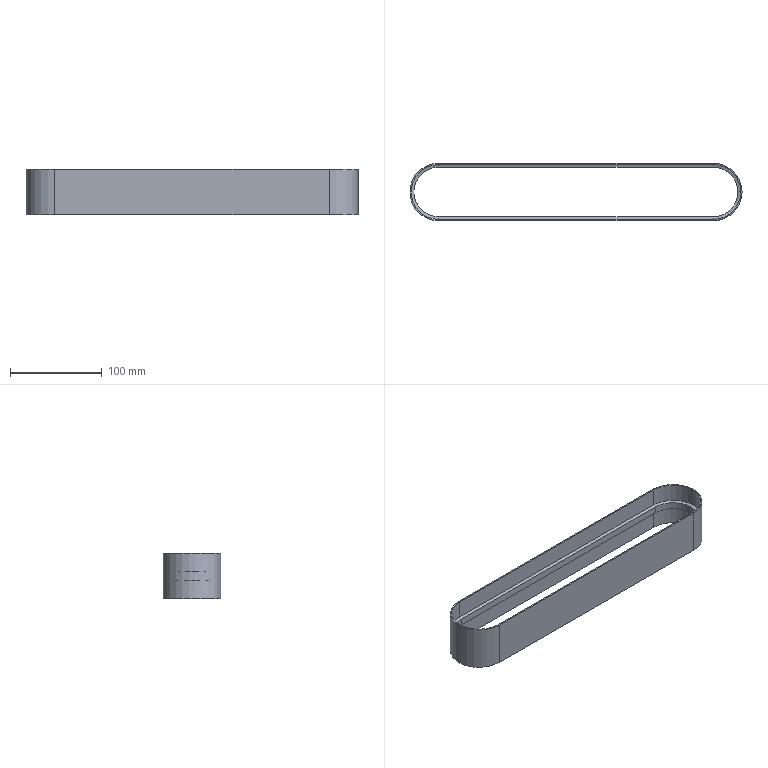Part | STEP file | EME01-W50-L0.793 flat belt Yihda 113 | 1 solid | 32 faces | box 362.8 x 62.8 x 50 mm | volume 76314 mm3 | plane 14 | cylinder 12 | cone 6 | commonest cylinder face diameters 60 x6 54 x3 62.8 x3
STEP:
#1=CARTESIAN_POINT('',(-150.,27.,-3.9));
#2=VERTEX_POINT('',#1);
#3=CARTESIAN_POINT('',(-177.,0.,-3.9));
#4=VERTEX_POINT('',#3);
#5=CARTESIAN_POINT('',(-150.,0.,-3.9));
#6=DIRECTION('',(0.,0.,1.));
#7=DIRECTION('',(1.,0.,0.));
#8=AXIS2_PLACEMENT_3D('',#5,#6,#7);
#9=CIRCLE('',#8,27.);
#10=EDGE_CURVE('',#2,#4,#9,.T.);
#11=ORIENTED_EDGE('',*,*,#10,.T.);
#12=CARTESIAN_POINT('',(-180.,0.,-5.));
#13=VERTEX_POINT('',#12);
#14=CARTESIAN_POINT('',(-177.,0.,-3.9));
#15=DIRECTION('',(-0.9389,0.,-0.3443));
#16=VECTOR('',#15,1000.);
#17=LINE('',#14,#16);
#18=EDGE_CURVE('',#4,#13,#17,.T.);
#19=ORIENTED_EDGE('',*,*,#18,.T.);
#20=CARTESIAN_POINT('',(-150.,30.,-5.));
#21=VERTEX_POINT('',#20);
#22=CARTESIAN_POINT('',(-150.,0.,-5.));
#23=DIRECTION('',(0.,0.,1.));
#24=DIRECTION('',(1.,0.,0.));
#25=AXIS2_PLACEMENT_3D('',#22,#23,#24);
#26=CIRCLE('',#25,30.);
#27=EDGE_CURVE('',#21,#13,#26,.T.);
#28=ORIENTED_EDGE('',*,*,#27,.F.);
#29=CARTESIAN_POINT('',(-150.,30.,-5.));
#30=DIRECTION('',(0.,0.9389,-0.3443));
#31=VECTOR('',#30,1000.);
#32=LINE('',#29,#31);
#33=EDGE_CURVE('',#2,#21,#32,.T.);
#34=ORIENTED_EDGE('',*,*,#33,.F.);
#35=EDGE_LOOP('',(#11,#19,#28,#34));
#36=FACE_OUTER_BOUND('',#35,.T.);
#37=CARTESIAN_POINT('',(-150.,0.,-3.9));
#38=DIRECTION('',(0.,0.,-1.));
#39=DIRECTION('',(-1.,0.,0.));
#40=AXIS2_PLACEMENT_3D('',#37,#38,#39);
#41=CONICAL_SURFACE('',#40,27.,1.219);
#42=ADVANCED_FACE('',(#36),#41,.F.);
#43=CARTESIAN_POINT('',(180.,0.,5.));
#44=VERTEX_POINT('',#43);
#45=CARTESIAN_POINT('',(150.,30.,5.));
#46=VERTEX_POINT('',#45);
#47=CARTESIAN_POINT('',(150.,0.,5.));
#48=DIRECTION('',(0.,0.,1.));
#49=DIRECTION('',(1.,0.,0.));
#50=AXIS2_PLACEMENT_3D('',#47,#48,#49);
#51=CIRCLE('',#50,30.);
#52=EDGE_CURVE('',#44,#46,#51,.T.);
#53=ORIENTED_EDGE('',*,*,#52,.F.);
#54=CARTESIAN_POINT('',(180.,0.,25.));
#55=VERTEX_POINT('',#54);
#56=CARTESIAN_POINT('',(180.,0.,0.));
#57=DIRECTION('',(0.,0.,1.));
#58=VECTOR('',#57,1000.);
#59=LINE('',#56,#58);
#60=EDGE_CURVE('',#44,#55,#59,.T.);
#61=ORIENTED_EDGE('',*,*,#60,.T.);
#62=CARTESIAN_POINT('',(150.,30.,25.));
#63=VERTEX_POINT('',#62);
#64=CARTESIAN_POINT('',(150.,0.,25.));
#65=DIRECTION('',(0.,0.,1.));
#66=DIRECTION('',(1.,0.,0.));
#67=AXIS2_PLACEMENT_3D('',#64,#65,#66);
#68=CIRCLE('',#67,30.);
#69=EDGE_CURVE('',#55,#63,#68,.T.);
#70=ORIENTED_EDGE('',*,*,#69,.T.);
#71=CARTESIAN_POINT('',(150.,30.,25.));
#72=DIRECTION('',(0.,0.,-1.));
#73=VECTOR('',#72,1000.);
#74=LINE('',#71,#73);
#75=EDGE_CURVE('',#63,#46,#74,.T.);
#76=ORIENTED_EDGE('',*,*,#75,.T.);
#77=EDGE_LOOP('',(#53,#61,#70,#76));
#78=FACE_OUTER_BOUND('',#77,.T.);
#79=CARTESIAN_POINT('',(150.,0.,0.));
#80=DIRECTION('',(0.,0.,1.));
#81=DIRECTION('',(1.,0.,0.));
#82=AXIS2_PLACEMENT_3D('',#79,#80,#81);
#83=CYLINDRICAL_SURFACE('',#82,30.);
#84=ADVANCED_FACE('',(#78),#83,.F.);
#85=CARTESIAN_POINT('',(177.,0.,3.9));
#86=VERTEX_POINT('',#85);
#87=CARTESIAN_POINT('',(150.,27.,3.9));
#88=VERTEX_POINT('',#87);
#89=CARTESIAN_POINT('',(150.,0.,3.9));
#90=DIRECTION('',(0.,0.,1.));
#91=DIRECTION('',(1.,0.,0.));
#92=AXIS2_PLACEMENT_3D('',#89,#90,#91);
#93=CIRCLE('',#92,27.);
#94=EDGE_CURVE('',#86,#88,#93,.T.);
#95=ORIENTED_EDGE('',*,*,#94,.F.);
#96=CARTESIAN_POINT('',(180.,0.,5.));
#97=DIRECTION('',(0.9389,0.,0.3443));
#98=VECTOR('',#97,1000.);
#99=LINE('',#96,#98);
#100=EDGE_CURVE('',#86,#44,#99,.T.);
#101=ORIENTED_EDGE('',*,*,#100,.T.);
#102=ORIENTED_EDGE('',*,*,#52,.T.);
#103=CARTESIAN_POINT('',(150.,30.,5.));
#104=DIRECTION('',(0.,-0.9389,-0.3443));
#105=VECTOR('',#104,1000.);
#106=LINE('',#103,#105);
#107=EDGE_CURVE('',#46,#88,#106,.T.);
#108=ORIENTED_EDGE('',*,*,#107,.T.);
#109=EDGE_LOOP('',(#95,#101,#102,#108));
#110=FACE_OUTER_BOUND('',#109,.T.);
#111=CARTESIAN_POINT('',(150.,0.,5.));
#112=DIRECTION('',(0.,0.,1.));
#113=DIRECTION('',(1.,0.,0.));
#114=AXIS2_PLACEMENT_3D('',#111,#112,#113);
#115=CONICAL_SURFACE('',#114,30.,1.219);
#116=ADVANCED_FACE('',(#110),#115,.F.);
#117=CARTESIAN_POINT('',(177.,0.,-3.9));
#118=VERTEX_POINT('',#117);
#119=CARTESIAN_POINT('',(150.,27.,-3.9));
#120=VERTEX_POINT('',#119);
#121=CARTESIAN_POINT('',(150.,0.,-3.9));
#122=DIRECTION('',(0.,0.,1.));
#123=DIRECTION('',(1.,0.,0.));
#124=AXIS2_PLACEMENT_3D('',#121,#122,#123);
#125=CIRCLE('',#124,27.);
#126=EDGE_CURVE('',#118,#120,#125,.T.);
#127=ORIENTED_EDGE('',*,*,#126,.F.);
#128=CARTESIAN_POINT('',(177.,0.,0.));
#129=DIRECTION('',(0.,0.,1.));
#130=VECTOR('',#129,1000.);
#131=LINE('',#128,#130);
#132=EDGE_CURVE('',#118,#86,#131,.T.);
#133=ORIENTED_EDGE('',*,*,#132,.T.);
#134=ORIENTED_EDGE('',*,*,#94,.T.);
#135=CARTESIAN_POINT('',(150.,27.,3.9));
#136=DIRECTION('',(0.,0.,-1.));
#137=VECTOR('',#136,1000.);
#138=LINE('',#135,#137);
#139=EDGE_CURVE('',#88,#120,#138,.T.);
#140=ORIENTED_EDGE('',*,*,#139,.T.);
#141=EDGE_LOOP('',(#127,#133,#134,#140));
#142=FACE_OUTER_BOUND('',#141,.T.);
#143=CARTESIAN_POINT('',(150.,0.,0.));
#144=DIRECTION('',(0.,0.,1.));
#145=DIRECTION('',(1.,0.,0.));
#146=AXIS2_PLACEMENT_3D('',#143,#144,#145);
#147=CYLINDRICAL_SURFACE('',#146,27.);
#148=ADVANCED_FACE('',(#142),#147,.F.);
#149=CARTESIAN_POINT('',(180.,0.,-25.));
#150=VERTEX_POINT('',#149);
#151=CARTESIAN_POINT('',(150.,30.,-25.));
#152=VERTEX_POINT('',#151);
#153=CARTESIAN_POINT('',(150.,0.,-25.));
#154=DIRECTION('',(0.,0.,1.));
#155=DIRECTION('',(1.,0.,0.));
#156=AXIS2_PLACEMENT_3D('',#153,#154,#155);
#157=CIRCLE('',#156,30.);
#158=EDGE_CURVE('',#150,#152,#157,.T.);
#159=ORIENTED_EDGE('',*,*,#158,.F.);
#160=CARTESIAN_POINT('',(180.,0.,-5.));
#161=VERTEX_POINT('',#160);
#162=CARTESIAN_POINT('',(180.,0.,0.));
#163=DIRECTION('',(0.,0.,1.));
#164=VECTOR('',#163,1000.);
#165=LINE('',#162,#164);
#166=EDGE_CURVE('',#150,#161,#165,.T.);
#167=ORIENTED_EDGE('',*,*,#166,.T.);
#168=CARTESIAN_POINT('',(150.,30.,-5.));
#169=VERTEX_POINT('',#168);
#170=CARTESIAN_POINT('',(150.,0.,-5.));
#171=DIRECTION('',(0.,0.,1.));
#172=DIRECTION('',(1.,0.,0.));
#173=AXIS2_PLACEMENT_3D('',#170,#171,#172);
#174=CIRCLE('',#173,30.);
#175=EDGE_CURVE('',#161,#169,#174,.T.);
#176=ORIENTED_EDGE('',*,*,#175,.T.);
#177=CARTESIAN_POINT('',(150.,30.,-5.));
#178=DIRECTION('',(0.,0.,-1.));
#179=VECTOR('',#178,1000.);
#180=LINE('',#177,#179);
#181=EDGE_CURVE('',#169,#152,#180,.T.);
#182=ORIENTED_EDGE('',*,*,#181,.T.);
#183=EDGE_LOOP('',(#159,#167,#176,#182));
#184=FACE_OUTER_BOUND('',#183,.T.);
#185=CARTESIAN_POINT('',(150.,0.,0.));
#186=DIRECTION('',(0.,0.,1.));
#187=DIRECTION('',(1.,0.,0.));
#188=AXIS2_PLACEMENT_3D('',#185,#186,#187);
#189=CYLINDRICAL_SURFACE('',#188,30.);
#190=ADVANCED_FACE('',(#184),#189,.F.);
#191=CARTESIAN_POINT('',(150.,-31.4,-25.));
#192=VERTEX_POINT('',#191);
#193=CARTESIAN_POINT('',(181.4,0.,-25.));
#194=VERTEX_POINT('',#193);
#195=CARTESIAN_POINT('',(150.,0.,-25.));
#196=DIRECTION('',(0.,0.,1.));
#197=DIRECTION('',(1.,0.,0.));
#198=AXIS2_PLACEMENT_3D('',#195,#196,#197);
#199=CIRCLE('',#198,31.4);
#200=EDGE_CURVE('',#192,#194,#199,.T.);
#201=ORIENTED_EDGE('',*,*,#200,.T.);
#202=CARTESIAN_POINT('',(181.4,0.,25.));
#203=VERTEX_POINT('',#202);
#204=CARTESIAN_POINT('',(181.4,0.,0.));
#205=DIRECTION('',(0.,0.,1.));
#206=VECTOR('',#205,1000.);
#207=LINE('',#204,#206);
#208=EDGE_CURVE('',#194,#203,#207,.T.);
#209=ORIENTED_EDGE('',*,*,#208,.T.);
#210=CARTESIAN_POINT('',(150.,-31.4,25.));
#211=VERTEX_POINT('',#210);
#212=CARTESIAN_POINT('',(150.,0.,25.));
#213=DIRECTION('',(0.,0.,1.));
#214=DIRECTION('',(1.,0.,0.));
#215=AXIS2_PLACEMENT_3D('',#212,#213,#214);
#216=CIRCLE('',#215,31.4);
#217=EDGE_CURVE('',#211,#203,#216,.T.);
#218=ORIENTED_EDGE('',*,*,#217,.F.);
#219=CARTESIAN_POINT('',(150.,-31.4,25.));
#220=DIRECTION('',(0.,0.,1.));
#221=VECTOR('',#220,1000.);
#222=LINE('',#219,#221);
#223=EDGE_CURVE('',#192,#211,#222,.T.);
#224=ORIENTED_EDGE('',*,*,#223,.F.);
#225=EDGE_LOOP('',(#201,#209,#218,#224));
#226=FACE_OUTER_BOUND('',#225,.T.);
#227=CARTESIAN_POINT('',(150.,0.,0.));
#228=DIRECTION('',(0.,0.,1.));
#229=DIRECTION('',(1.,0.,0.));
#230=AXIS2_PLACEMENT_3D('',#227,#228,#229);
#231=CYLINDRICAL_SURFACE('',#230,31.4);
#232=ADVANCED_FACE('',(#226),#231,.T.);
#233=ORIENTED_EDGE('',*,*,#208,.F.);
#234=CARTESIAN_POINT('',(150.,31.4,-25.));
#235=VERTEX_POINT('',#234);
#236=CARTESIAN_POINT('',(150.,0.,-25.));
#237=DIRECTION('',(0.,0.,1.));
#238=DIRECTION('',(1.,0.,0.));
#239=AXIS2_PLACEMENT_3D('',#236,#237,#238);
#240=CIRCLE('',#239,31.4);
#241=EDGE_CURVE('',#194,#235,#240,.T.);
#242=ORIENTED_EDGE('',*,*,#241,.T.);
#243=CARTESIAN_POINT('',(150.,31.4,25.));
#244=VERTEX_POINT('',#243);
#245=CARTESIAN_POINT('',(150.,31.4,25.));
#246=DIRECTION('',(0.,0.,1.));
#247=VECTOR('',#246,1000.);
#248=LINE('',#245,#247);
#249=EDGE_CURVE('',#235,#244,#248,.T.);
#250=ORIENTED_EDGE('',*,*,#249,.T.);
#251=CARTESIAN_POINT('',(150.,0.,25.));
#252=DIRECTION('',(0.,0.,1.));
#253=DIRECTION('',(1.,0.,0.));
#254=AXIS2_PLACEMENT_3D('',#251,#252,#253);
#255=CIRCLE('',#254,31.4);
#256=EDGE_CURVE('',#203,#244,#255,.T.);
#257=ORIENTED_EDGE('',*,*,#256,.F.);
#258=EDGE_LOOP('',(#233,#242,#250,#257));
#259=FACE_OUTER_BOUND('',#258,.T.);
#260=CARTESIAN_POINT('',(150.,0.,0.));
#261=DIRECTION('',(0.,0.,1.));
#262=DIRECTION('',(1.,0.,0.));
#263=AXIS2_PLACEMENT_3D('',#260,#261,#262);
#264=CYLINDRICAL_SURFACE('',#263,31.4);
#265=ADVANCED_FACE('',(#259),#264,.T.);
#266=ORIENTED_EDGE('',*,*,#166,.F.);
#267=CARTESIAN_POINT('',(150.,-30.,-25.));
#268=VERTEX_POINT('',#267);
#269=CARTESIAN_POINT('',(150.,0.,-25.));
#270=DIRECTION('',(0.,0.,1.));
#271=DIRECTION('',(1.,0.,0.));
#272=AXIS2_PLACEMENT_3D('',#269,#270,#271);
#273=CIRCLE('',#272,30.);
#274=EDGE_CURVE('',#268,#150,#273,.T.);
#275=ORIENTED_EDGE('',*,*,#274,.F.);
#276=CARTESIAN_POINT('',(150.,-30.,-5.));
#277=VERTEX_POINT('',#276);
#278=CARTESIAN_POINT('',(150.,-30.,-5.));
#279=DIRECTION('',(0.,0.,-1.));
#280=VECTOR('',#279,1000.);
#281=LINE('',#278,#280);
#282=EDGE_CURVE('',#277,#268,#281,.T.);
#283=ORIENTED_EDGE('',*,*,#282,.F.);
#284=CARTESIAN_POINT('',(150.,0.,-5.));
#285=DIRECTION('',(0.,0.,1.));
#286=DIRECTION('',(1.,0.,0.));
#287=AXIS2_PLACEMENT_3D('',#284,#285,#286);
#288=CIRCLE('',#287,30.);
#289=EDGE_CURVE('',#277,#161,#288,.T.);
#290=ORIENTED_EDGE('',*,*,#289,.T.);
#291=EDGE_LOOP('',(#266,#275,#283,#290));
#292=FACE_OUTER_BOUND('',#291,.T.);
#293=CARTESIAN_POINT('',(150.,0.,0.));
#294=DIRECTION('',(0.,0.,1.));
#295=DIRECTION('',(1.,0.,0.));
#296=AXIS2_PLACEMENT_3D('',#293,#294,#295);
#297=CYLINDRICAL_SURFACE('',#296,30.);
#298=ADVANCED_FACE('',(#292),#297,.F.);
#299=CARTESIAN_POINT('',(150.,-27.,-3.9));
#300=VERTEX_POINT('',#299);
#301=CARTESIAN_POINT('',(150.,-30.,-5.));
#302=DIRECTION('',(0.,-0.9389,-0.3443));
#303=VECTOR('',#302,1000.);
#304=LINE('',#301,#303);
#305=EDGE_CURVE('',#300,#277,#304,.T.);
#306=ORIENTED_EDGE('',*,*,#305,.F.);
#307=CARTESIAN_POINT('',(150.,0.,-3.9));
#308=DIRECTION('',(0.,0.,1.));
#309=DIRECTION('',(1.,0.,0.));
#310=AXIS2_PLACEMENT_3D('',#307,#308,#309);
#311=CIRCLE('',#310,27.);
#312=EDGE_CURVE('',#300,#118,#311,.T.);
#313=ORIENTED_EDGE('',*,*,#312,.T.);
#314=ORIENTED_EDGE('',*,*,#126,.T.);
#315=CARTESIAN_POINT('',(150.,30.,-5.));
#316=DIRECTION('',(0.,0.9389,-0.3443));
#317=VECTOR('',#316,1000.);
#318=LINE('',#315,#317);
#319=EDGE_CURVE('',#120,#169,#318,.T.);
#320=ORIENTED_EDGE('',*,*,#319,.T.);
#321=ORIENTED_EDGE('',*,*,#175,.F.);
#322=ORIENTED_EDGE('',*,*,#289,.F.);
#323=EDGE_LOOP('',(#306,#313,#314,#320,#321,#322));
#324=FACE_OUTER_BOUND('',#323,.T.);
#325=CARTESIAN_POINT('',(150.,0.,-3.9));
#326=DIRECTION('',(0.,0.,-1.));
#327=DIRECTION('',(-1.,0.,0.));
#328=AXIS2_PLACEMENT_3D('',#325,#326,#327);
#329=CONICAL_SURFACE('',#328,27.,1.219);
#330=ADVANCED_FACE('',(#324),#329,.F.);
#331=ORIENTED_EDGE('',*,*,#132,.F.);
#332=ORIENTED_EDGE('',*,*,#312,.F.);
#333=CARTESIAN_POINT('',(150.,-27.,3.9));
#334=VERTEX_POINT('',#333);
#335=CARTESIAN_POINT('',(150.,-27.,3.9));
#336=DIRECTION('',(0.,0.,-1.));
#337=VECTOR('',#336,1000.);
#338=LINE('',#335,#337);
#339=EDGE_CURVE('',#334,#300,#338,.T.);
#340=ORIENTED_EDGE('',*,*,#339,.F.);
#341=CARTESIAN_POINT('',(150.,0.,3.9));
#342=DIRECTION('',(0.,0.,1.));
#343=DIRECTION('',(1.,0.,0.));
#344=AXIS2_PLACEMENT_3D('',#341,#342,#343);
#345=CIRCLE('',#344,27.);
#346=EDGE_CURVE('',#334,#86,#345,.T.);
#347=ORIENTED_EDGE('',*,*,#346,.T.);
#348=EDGE_LOOP('',(#331,#332,#340,#347));
#349=FACE_OUTER_BOUND('',#348,.T.);
#350=CARTESIAN_POINT('',(150.,0.,0.));
#351=DIRECTION('',(0.,0.,1.));
#352=DIRECTION('',(1.,0.,0.));
#353=AXIS2_PLACEMENT_3D('',#350,#351,#352);
#354=CYLINDRICAL_SURFACE('',#353,27.);
#355=ADVANCED_FACE('',(#349),#354,.F.);
#356=ORIENTED_EDGE('',*,*,#100,.F.);
#357=ORIENTED_EDGE('',*,*,#346,.F.);
#358=CARTESIAN_POINT('',(150.,-30.,5.));
#359=VERTEX_POINT('',#358);
#360=CARTESIAN_POINT('',(150.,-30.,5.));
#361=DIRECTION('',(0.,0.9389,-0.3443));
#362=VECTOR('',#361,1000.);
#363=LINE('',#360,#362);
#364=EDGE_CURVE('',#359,#334,#363,.T.);
#365=ORIENTED_EDGE('',*,*,#364,.F.);
#366=CARTESIAN_POINT('',(150.,0.,5.));
#367=DIRECTION('',(0.,0.,1.));
#368=DIRECTION('',(1.,0.,0.));
#369=AXIS2_PLACEMENT_3D('',#366,#367,#368);
#370=CIRCLE('',#369,30.);
#371=EDGE_CURVE('',#359,#44,#370,.T.);
#372=ORIENTED_EDGE('',*,*,#371,.T.);
#373=EDGE_LOOP('',(#356,#357,#365,#372));
#374=FACE_OUTER_BOUND('',#373,.T.);
#375=CARTESIAN_POINT('',(150.,0.,5.));
#376=DIRECTION('',(0.,0.,1.));
#377=DIRECTION('',(1.,0.,0.));
#378=AXIS2_PLACEMENT_3D('',#375,#376,#377);
#379=CONICAL_SURFACE('',#378,30.,1.219);
#380=ADVANCED_FACE('',(#374),#379,.F.);
#381=ORIENTED_EDGE('',*,*,#60,.F.);
#382=ORIENTED_EDGE('',*,*,#371,.F.);
#383=CARTESIAN_POINT('',(150.,-30.,25.));
#384=VERTEX_POINT('',#383);
#385=CARTESIAN_POINT('',(150.,-30.,25.));
#386=DIRECTION('',(0.,0.,-1.));
#387=VECTOR('',#386,1000.);
#388=LINE('',#385,#387);
#389=EDGE_CURVE('',#384,#359,#388,.T.);
#390=ORIENTED_EDGE('',*,*,#389,.F.);
#391=CARTESIAN_POINT('',(150.,0.,25.));
#392=DIRECTION('',(0.,0.,1.));
#393=DIRECTION('',(1.,0.,0.));
#394=AXIS2_PLACEMENT_3D('',#391,#392,#393);
#395=CIRCLE('',#394,30.);
#396=EDGE_CURVE('',#384,#55,#395,.T.);
#397=ORIENTED_EDGE('',*,*,#396,.T.);
#398=EDGE_LOOP('',(#381,#382,#390,#397));
#399=FACE_OUTER_BOUND('',#398,.T.);
#400=CARTESIAN_POINT('',(150.,0.,0.));
#401=DIRECTION('',(0.,0.,1.));
#402=DIRECTION('',(1.,0.,0.));
#403=AXIS2_PLACEMENT_3D('',#400,#401,#402);
#404=CYLINDRICAL_SURFACE('',#403,30.);
#405=ADVANCED_FACE('',(#399),#404,.F.);
#406=CARTESIAN_POINT('',(-150.,-31.4,-25.));
#407=VERTEX_POINT('',#406);
#408=CARTESIAN_POINT('',(-150.,-31.4,25.));
#409=VERTEX_POINT('',#408);
#410=CARTESIAN_POINT('',(-150.,-31.4,25.));
#411=DIRECTION('',(0.,0.,1.));
#412=VECTOR('',#411,1000.);
#413=LINE('',#410,#412);
#414=EDGE_CURVE('',#407,#409,#413,.T.);
#415=ORIENTED_EDGE('',*,*,#414,.F.);
#416=CARTESIAN_POINT('',(-150.,-31.4,-25.));
#417=DIRECTION('',(1.,0.,0.));
#418=VECTOR('',#417,1000.);
#419=LINE('',#416,#418);
#420=EDGE_CURVE('',#407,#192,#419,.T.);
#421=ORIENTED_EDGE('',*,*,#420,.T.);
#422=ORIENTED_EDGE('',*,*,#223,.T.);
#423=CARTESIAN_POINT('',(-150.,-31.4,25.));
#424=DIRECTION('',(1.,0.,0.));
#425=VECTOR('',#424,1000.);
#426=LINE('',#423,#425);
#427=EDGE_CURVE('',#409,#211,#426,.T.);
#428=ORIENTED_EDGE('',*,*,#427,.F.);
#429=EDGE_LOOP('',(#415,#421,#422,#428));
#430=FACE_OUTER_BOUND('',#429,.T.);
#431=CARTESIAN_POINT('',(-150.,-31.4,25.));
#432=DIRECTION('',(0.,1.,0.));
#433=DIRECTION('',(-1.,0.,0.));
#434=AXIS2_PLACEMENT_3D('',#431,#432,#433);
#435=PLANE('',#434);
#436=ADVANCED_FACE('',(#430),#435,.F.);
#437=CARTESIAN_POINT('',(-150.,-30.,-5.));
#438=VERTEX_POINT('',#437);
#439=CARTESIAN_POINT('',(-150.,-30.,-25.));
#440=VERTEX_POINT('',#439);
#441=CARTESIAN_POINT('',(-150.,-30.,-5.));
#442=DIRECTION('',(0.,0.,-1.));
#443=VECTOR('',#442,1000.);
#444=LINE('',#441,#443);
#445=EDGE_CURVE('',#438,#440,#444,.T.);
#446=ORIENTED_EDGE('',*,*,#445,.F.);
#447=CARTESIAN_POINT('',(-150.,-30.,-5.));
#448=DIRECTION('',(1.,0.,0.));
#449=VECTOR('',#448,1000.);
#450=LINE('',#447,#449);
#451=EDGE_CURVE('',#438,#277,#450,.T.);
#452=ORIENTED_EDGE('',*,*,#451,.T.);
#453=ORIENTED_EDGE('',*,*,#282,.T.);
#454=CARTESIAN_POINT('',(-150.,-30.,-25.));
#455=DIRECTION('',(1.,0.,0.));
#456=VECTOR('',#455,1000.);
#457=LINE('',#454,#456);
#458=EDGE_CURVE('',#440,#268,#457,.T.);
#459=ORIENTED_EDGE('',*,*,#458,.F.);
#460=EDGE_LOOP('',(#446,#452,#453,#459));
#461=FACE_OUTER_BOUND('',#460,.T.);
#462=CARTESIAN_POINT('',(-150.,-30.,-5.));
#463=DIRECTION('',(0.,-1.,0.));
#464=DIRECTION('',(1.,0.,0.));
#465=AXIS2_PLACEMENT_3D('',#462,#463,#464);
#466=PLANE('',#465);
#467=ADVANCED_FACE('',(#461),#466,.F.);
#468=CARTESIAN_POINT('',(-150.,-27.,-3.9));
#469=VERTEX_POINT('',#468);
#470=CARTESIAN_POINT('',(-150.,-30.,-5.));
#471=DIRECTION('',(0.,-0.9389,-0.3443));
#472=VECTOR('',#471,1000.);
#473=LINE('',#470,#472);
#474=EDGE_CURVE('',#469,#438,#473,.T.);
#475=ORIENTED_EDGE('',*,*,#474,.F.);
#476=CARTESIAN_POINT('',(-150.,-27.,-3.9));
#477=DIRECTION('',(1.,0.,0.));
#478=VECTOR('',#477,1000.);
#479=LINE('',#476,#478);
#480=EDGE_CURVE('',#469,#300,#479,.T.);
#481=ORIENTED_EDGE('',*,*,#480,.T.);
#482=ORIENTED_EDGE('',*,*,#305,.T.);
#483=ORIENTED_EDGE('',*,*,#451,.F.);
#484=EDGE_LOOP('',(#475,#481,#482,#483));
#485=FACE_OUTER_BOUND('',#484,.T.);
#486=CARTESIAN_POINT('',(-150.,-30.,-5.));
#487=DIRECTION('',(0.,-0.3443,0.9389));
#488=DIRECTION('',(0.,-0.9389,-0.3443));
#489=AXIS2_PLACEMENT_3D('',#486,#487,#488);
#490=PLANE('',#489);
#491=ADVANCED_FACE('',(#485),#490,.F.);
#492=CARTESIAN_POINT('',(-150.,-27.,3.9));
#493=VERTEX_POINT('',#492);
#494=CARTESIAN_POINT('',(-150.,-27.,3.9));
#495=DIRECTION('',(0.,0.,-1.));
#496=VECTOR('',#495,1000.);
#497=LINE('',#494,#496);
#498=EDGE_CURVE('',#493,#469,#497,.T.);
#499=ORIENTED_EDGE('',*,*,#498,.F.);
#500=CARTESIAN_POINT('',(-150.,-27.,3.9));
#501=DIRECTION('',(1.,0.,0.));
#502=VECTOR('',#501,1000.);
#503=LINE('',#500,#502);
#504=EDGE_CURVE('',#493,#334,#503,.T.);
#505=ORIENTED_EDGE('',*,*,#504,.T.);
#506=ORIENTED_EDGE('',*,*,#339,.T.);
#507=ORIENTED_EDGE('',*,*,#480,.F.);
#508=EDGE_LOOP('',(#499,#505,#506,#507));
#509=FACE_OUTER_BOUND('',#508,.T.);
#510=CARTESIAN_POINT('',(-150.,-27.,3.9));
#511=DIRECTION('',(0.,-1.,0.));
#512=DIRECTION('',(1.,0.,0.));
#513=AXIS2_PLACEMENT_3D('',#510,#511,#512);
#514=PLANE('',#513);
#515=ADVANCED_FACE('',(#509),#514,.F.);
#516=CARTESIAN_POINT('',(-150.,-30.,5.));
#517=VERTEX_POINT('',#516);
#518=CARTESIAN_POINT('',(-150.,-30.,5.));
#519=DIRECTION('',(0.,0.9389,-0.3443));
#520=VECTOR('',#519,1000.);
#521=LINE('',#518,#520);
#522=EDGE_CURVE('',#517,#493,#521,.T.);
#523=ORIENTED_EDGE('',*,*,#522,.F.);
#524=CARTESIAN_POINT('',(-150.,-30.,5.));
#525=DIRECTION('',(1.,0.,0.));
#526=VECTOR('',#525,1000.);
#527=LINE('',#524,#526);
#528=EDGE_CURVE('',#517,#359,#527,.T.);
#529=ORIENTED_EDGE('',*,*,#528,.T.);
#530=ORIENTED_EDGE('',*,*,#364,.T.);
#531=ORIENTED_EDGE('',*,*,#504,.F.);
#532=EDGE_LOOP('',(#523,#529,#530,#531));
#533=FACE_OUTER_BOUND('',#532,.T.);
#534=CARTESIAN_POINT('',(-150.,-30.,5.));
#535=DIRECTION('',(0.,-0.3443,-0.9389));
#536=DIRECTION('',(0.,0.9389,-0.3443));
#537=AXIS2_PLACEMENT_3D('',#534,#535,#536);
#538=PLANE('',#537);
#539=ADVANCED_FACE('',(#533),#538,.F.);
#540=CARTESIAN_POINT('',(-150.,-30.,25.));
#541=VERTEX_POINT('',#540);
#542=CARTESIAN_POINT('',(-150.,-30.,25.));
#543=DIRECTION('',(0.,0.,-1.));
#544=VECTOR('',#543,1000.);
#545=LINE('',#542,#544);
#546=EDGE_CURVE('',#541,#517,#545,.T.);
#547=ORIENTED_EDGE('',*,*,#546,.F.);
#548=CARTESIAN_POINT('',(-150.,-30.,25.));
#549=DIRECTION('',(1.,0.,0.));
#550=VECTOR('',#549,1000.);
#551=LINE('',#548,#550);
#552=EDGE_CURVE('',#541,#384,#551,.T.);
#553=ORIENTED_EDGE('',*,*,#552,.T.);
#554=ORIENTED_EDGE('',*,*,#389,.T.);
#555=ORIENTED_EDGE('',*,*,#528,.F.);
#556=EDGE_LOOP('',(#547,#553,#554,#555));
#557=FACE_OUTER_BOUND('',#556,.T.);
#558=CARTESIAN_POINT('',(-150.,-30.,25.));
#559=DIRECTION('',(0.,-1.,0.));
#560=DIRECTION('',(1.,0.,0.));
#561=AXIS2_PLACEMENT_3D('',#558,#559,#560);
#562=PLANE('',#561);
#563=ADVANCED_FACE('',(#557),#562,.F.);
#564=CARTESIAN_POINT('',(-150.,31.4,-25.));
#565=VERTEX_POINT('',#564);
#566=CARTESIAN_POINT('',(-150.,31.4,25.));
#567=VERTEX_POINT('',#566);
#568=CARTESIAN_POINT('',(-150.,31.4,25.));
#569=DIRECTION('',(0.,0.,1.));
#570=VECTOR('',#569,1000.);
#571=LINE('',#568,#570);
#572=EDGE_CURVE('',#565,#567,#571,.T.);
#573=ORIENTED_EDGE('',*,*,#572,.F.);
#574=CARTESIAN_POINT('',(-150.,0.,-25.));
#575=DIRECTION('',(0.,0.,1.));
#576=DIRECTION('',(1.,0.,0.));
#577=AXIS2_PLACEMENT_3D('',#574,#575,#576);
#578=CIRCLE('',#577,31.4);
#579=EDGE_CURVE('',#565,#407,#578,.T.);
#580=ORIENTED_EDGE('',*,*,#579,.T.);
#581=ORIENTED_EDGE('',*,*,#414,.T.);
#582=CARTESIAN_POINT('',(-150.,0.,25.));
#583=DIRECTION('',(0.,0.,1.));
#584=DIRECTION('',(1.,0.,0.));
#585=AXIS2_PLACEMENT_3D('',#582,#583,#584);
#586=CIRCLE('',#585,31.4);
#587=EDGE_CURVE('',#567,#409,#586,.T.);
#588=ORIENTED_EDGE('',*,*,#587,.F.);
#589=EDGE_LOOP('',(#573,#580,#581,#588));
#590=FACE_OUTER_BOUND('',#589,.T.);
#591=CARTESIAN_POINT('',(-150.,0.,0.));
#592=DIRECTION('',(0.,0.,1.));
#593=DIRECTION('',(1.,0.,0.));
#594=AXIS2_PLACEMENT_3D('',#591,#592,#593);
#595=CYLINDRICAL_SURFACE('',#594,31.4);
#596=ADVANCED_FACE('',(#590),#595,.T.);
#597=CARTESIAN_POINT('',(-150.,30.,-25.));
#598=VERTEX_POINT('',#597);
#599=CARTESIAN_POINT('',(-150.,30.,-5.));
#600=DIRECTION('',(0.,0.,-1.));
#601=VECTOR('',#600,1000.);
#602=LINE('',#599,#601);
#603=EDGE_CURVE('',#21,#598,#602,.T.);
#604=ORIENTED_EDGE('',*,*,#603,.F.);
#605=ORIENTED_EDGE('',*,*,#27,.T.);
#606=CARTESIAN_POINT('',(-150.,0.,-5.));
#607=DIRECTION('',(0.,0.,1.));
#608=DIRECTION('',(1.,0.,0.));
#609=AXIS2_PLACEMENT_3D('',#606,#607,#608);
#610=CIRCLE('',#609,30.);
#611=EDGE_CURVE('',#13,#438,#610,.T.);
#612=ORIENTED_EDGE('',*,*,#611,.T.);
#613=ORIENTED_EDGE('',*,*,#445,.T.);
#614=CARTESIAN_POINT('',(-150.,0.,-25.));
#615=DIRECTION('',(0.,0.,1.));
#616=DIRECTION('',(1.,0.,0.));
#617=AXIS2_PLACEMENT_3D('',#614,#615,#616);
#618=CIRCLE('',#617,30.);
#619=EDGE_CURVE('',#598,#440,#618,.T.);
#620=ORIENTED_EDGE('',*,*,#619,.F.);
#621=EDGE_LOOP('',(#604,#605,#612,#613,#620));
#622=FACE_OUTER_BOUND('',#621,.T.);
#623=CARTESIAN_POINT('',(-150.,0.,0.));
#624=DIRECTION('',(0.,0.,1.));
#625=DIRECTION('',(1.,0.,0.));
#626=AXIS2_PLACEMENT_3D('',#623,#624,#625);
#627=CYLINDRICAL_SURFACE('',#626,30.);
#628=ADVANCED_FACE('',(#622),#627,.F.);
#629=ORIENTED_EDGE('',*,*,#18,.F.);
#630=CARTESIAN_POINT('',(-150.,0.,-3.9));
#631=DIRECTION('',(0.,0.,1.));
#632=DIRECTION('',(1.,0.,0.));
#633=AXIS2_PLACEMENT_3D('',#630,#631,#632);
#634=CIRCLE('',#633,27.);
#635=EDGE_CURVE('',#4,#469,#634,.T.);
#636=ORIENTED_EDGE('',*,*,#635,.T.);
#637=ORIENTED_EDGE('',*,*,#474,.T.);
#638=ORIENTED_EDGE('',*,*,#611,.F.);
#639=EDGE_LOOP('',(#629,#636,#637,#638));
#640=FACE_OUTER_BOUND('',#639,.T.);
#641=CARTESIAN_POINT('',(-150.,0.,-3.9));
#642=DIRECTION('',(0.,0.,-1.));
#643=DIRECTION('',(-1.,0.,0.));
#644=AXIS2_PLACEMENT_3D('',#641,#642,#643);
#645=CONICAL_SURFACE('',#644,27.,1.219);
#646=ADVANCED_FACE('',(#640),#645,.F.);
#647=CARTESIAN_POINT('',(-150.,27.,3.9));
#648=VERTEX_POINT('',#647);
#649=CARTESIAN_POINT('',(-150.,27.,3.9));
#650=DIRECTION('',(0.,0.,-1.));
#651=VECTOR('',#650,1000.);
#652=LINE('',#649,#651);
#653=EDGE_CURVE('',#648,#2,#652,.T.);
#654=ORIENTED_EDGE('',*,*,#653,.F.);
#655=CARTESIAN_POINT('',(-150.,0.,3.9));
#656=DIRECTION('',(0.,0.,1.));
#657=DIRECTION('',(1.,0.,0.));
#658=AXIS2_PLACEMENT_3D('',#655,#656,#657);
#659=CIRCLE('',#658,27.);
#660=EDGE_CURVE('',#648,#493,#659,.T.);
#661=ORIENTED_EDGE('',*,*,#660,.T.);
#662=ORIENTED_EDGE('',*,*,#498,.T.);
#663=ORIENTED_EDGE('',*,*,#635,.F.);
#664=ORIENTED_EDGE('',*,*,#10,.F.);
#665=EDGE_LOOP('',(#654,#661,#662,#663,#664));
#666=FACE_OUTER_BOUND('',#665,.T.);
#667=CARTESIAN_POINT('',(-150.,0.,0.));
#668=DIRECTION('',(0.,0.,1.));
#669=DIRECTION('',(1.,0.,0.));
#670=AXIS2_PLACEMENT_3D('',#667,#668,#669);
#671=CYLINDRICAL_SURFACE('',#670,27.);
#672=ADVANCED_FACE('',(#666),#671,.F.);
#673=CARTESIAN_POINT('',(-150.,30.,5.));
#674=VERTEX_POINT('',#673);
#675=CARTESIAN_POINT('',(-150.,30.,5.));
#676=DIRECTION('',(0.,-0.9389,-0.3443));
#677=VECTOR('',#676,1000.);
#678=LINE('',#675,#677);
#679=EDGE_CURVE('',#674,#648,#678,.T.);
#680=ORIENTED_EDGE('',*,*,#679,.F.);
#681=CARTESIAN_POINT('',(-150.,0.,5.));
#682=DIRECTION('',(0.,0.,1.));
#683=DIRECTION('',(1.,0.,0.));
#684=AXIS2_PLACEMENT_3D('',#681,#682,#683);
#685=CIRCLE('',#684,30.);
#686=EDGE_CURVE('',#674,#517,#685,.T.);
#687=ORIENTED_EDGE('',*,*,#686,.T.);
#688=ORIENTED_EDGE('',*,*,#522,.T.);
#689=ORIENTED_EDGE('',*,*,#660,.F.);
#690=EDGE_LOOP('',(#680,#687,#688,#689));
#691=FACE_OUTER_BOUND('',#690,.T.);
#692=CARTESIAN_POINT('',(-150.,0.,5.));
#693=DIRECTION('',(0.,0.,1.));
#694=DIRECTION('',(1.,0.,0.));
#695=AXIS2_PLACEMENT_3D('',#692,#693,#694);
#696=CONICAL_SURFACE('',#695,30.,1.219);
#697=ADVANCED_FACE('',(#691),#696,.F.);
#698=CARTESIAN_POINT('',(-150.,30.,25.));
#699=VERTEX_POINT('',#698);
#700=CARTESIAN_POINT('',(-150.,30.,25.));
#701=DIRECTION('',(0.,0.,-1.));
#702=VECTOR('',#701,1000.);
#703=LINE('',#700,#702);
#704=EDGE_CURVE('',#699,#674,#703,.T.);
#705=ORIENTED_EDGE('',*,*,#704,.F.);
#706=CARTESIAN_POINT('',(-150.,0.,25.));
#707=DIRECTION('',(0.,0.,1.));
#708=DIRECTION('',(1.,0.,0.));
#709=AXIS2_PLACEMENT_3D('',#706,#707,#708);
#710=CIRCLE('',#709,30.);
#711=EDGE_CURVE('',#699,#541,#710,.T.);
#712=ORIENTED_EDGE('',*,*,#711,.T.);
#713=ORIENTED_EDGE('',*,*,#546,.T.);
#714=ORIENTED_EDGE('',*,*,#686,.F.);
#715=EDGE_LOOP('',(#705,#712,#713,#714));
#716=FACE_OUTER_BOUND('',#715,.T.);
#717=CARTESIAN_POINT('',(-150.,0.,0.));
#718=DIRECTION('',(0.,0.,1.));
#719=DIRECTION('',(1.,0.,0.));
#720=AXIS2_PLACEMENT_3D('',#717,#718,#719);
#721=CYLINDRICAL_SURFACE('',#720,30.);
#722=ADVANCED_FACE('',(#716),#721,.F.);
#723=ORIENTED_EDGE('',*,*,#711,.F.);
#724=CARTESIAN_POINT('',(-150.,30.,25.));
#725=DIRECTION('',(1.,0.,0.));
#726=VECTOR('',#725,1000.);
#727=LINE('',#724,#726);
#728=EDGE_CURVE('',#699,#63,#727,.T.);
#729=ORIENTED_EDGE('',*,*,#728,.T.);
#730=ORIENTED_EDGE('',*,*,#69,.F.);
#731=ORIENTED_EDGE('',*,*,#396,.F.);
#732=ORIENTED_EDGE('',*,*,#552,.F.);
#733=EDGE_LOOP('',(#723,#729,#730,#731,#732));
#734=FACE_BOUND('',#733,.T.);
#735=CARTESIAN_POINT('',(-150.,31.4,25.));
#736=DIRECTION('',(1.,0.,0.));
#737=VECTOR('',#736,1000.);
#738=LINE('',#735,#737);
#739=EDGE_CURVE('',#567,#244,#738,.T.);
#740=ORIENTED_EDGE('',*,*,#739,.F.);
#741=ORIENTED_EDGE('',*,*,#587,.T.);
#742=ORIENTED_EDGE('',*,*,#427,.T.);
#743=ORIENTED_EDGE('',*,*,#217,.T.);
#744=ORIENTED_EDGE('',*,*,#256,.T.);
#745=EDGE_LOOP('',(#740,#741,#742,#743,#744));
#746=FACE_OUTER_BOUND('',#745,.T.);
#747=CARTESIAN_POINT('',(-150.,30.,25.));
#748=DIRECTION('',(0.,0.,1.));
#749=DIRECTION('',(1.,0.,0.));
#750=AXIS2_PLACEMENT_3D('',#747,#748,#749);
#751=PLANE('',#750);
#752=ADVANCED_FACE('',(#734,#746),#751,.T.);
#753=ORIENTED_EDGE('',*,*,#739,.T.);
#754=ORIENTED_EDGE('',*,*,#249,.F.);
#755=CARTESIAN_POINT('',(-150.,31.4,-25.));
#756=DIRECTION('',(1.,0.,0.));
#757=VECTOR('',#756,1000.);
#758=LINE('',#755,#757);
#759=EDGE_CURVE('',#565,#235,#758,.T.);
#760=ORIENTED_EDGE('',*,*,#759,.F.);
#761=ORIENTED_EDGE('',*,*,#572,.T.);
#762=EDGE_LOOP('',(#753,#754,#760,#761));
#763=FACE_OUTER_BOUND('',#762,.T.);
#764=CARTESIAN_POINT('',(-150.,31.4,25.));
#765=DIRECTION('',(0.,1.,0.));
#766=DIRECTION('',(0.,0.,1.));
#767=AXIS2_PLACEMENT_3D('',#764,#765,#766);
#768=PLANE('',#767);
#769=ADVANCED_FACE('',(#763),#768,.T.);
#770=ORIENTED_EDGE('',*,*,#579,.F.);
#771=ORIENTED_EDGE('',*,*,#759,.T.);
#772=ORIENTED_EDGE('',*,*,#241,.F.);
#773=ORIENTED_EDGE('',*,*,#200,.F.);
#774=ORIENTED_EDGE('',*,*,#420,.F.);
#775=EDGE_LOOP('',(#770,#771,#772,#773,#774));
#776=FACE_OUTER_BOUND('',#775,.T.);
#777=CARTESIAN_POINT('',(-150.,30.,-25.));
#778=DIRECTION('',(1.,0.,0.));
#779=VECTOR('',#778,1000.);
#780=LINE('',#777,#779);
#781=EDGE_CURVE('',#598,#152,#780,.T.);
#782=ORIENTED_EDGE('',*,*,#781,.F.);
#783=ORIENTED_EDGE('',*,*,#619,.T.);
#784=ORIENTED_EDGE('',*,*,#458,.T.);
#785=ORIENTED_EDGE('',*,*,#274,.T.);
#786=ORIENTED_EDGE('',*,*,#158,.T.);
#787=EDGE_LOOP('',(#782,#783,#784,#785,#786));
#788=FACE_BOUND('',#787,.T.);
#789=CARTESIAN_POINT('',(-150.,31.4,-25.));
#790=DIRECTION('',(0.,0.,-1.));
#791=DIRECTION('',(-1.,0.,0.));
#792=AXIS2_PLACEMENT_3D('',#789,#790,#791);
#793=PLANE('',#792);
#794=ADVANCED_FACE('',(#776,#788),#793,.T.);
#795=ORIENTED_EDGE('',*,*,#781,.T.);
#796=ORIENTED_EDGE('',*,*,#181,.F.);
#797=CARTESIAN_POINT('',(-150.,30.,-5.));
#798=DIRECTION('',(1.,0.,0.));
#799=VECTOR('',#798,1000.);
#800=LINE('',#797,#799);
#801=EDGE_CURVE('',#21,#169,#800,.T.);
#802=ORIENTED_EDGE('',*,*,#801,.F.);
#803=ORIENTED_EDGE('',*,*,#603,.T.);
#804=EDGE_LOOP('',(#795,#796,#802,#803));
#805=FACE_OUTER_BOUND('',#804,.T.);
#806=CARTESIAN_POINT('',(-150.,30.,-5.));
#807=DIRECTION('',(0.,-1.,0.));
#808=DIRECTION('',(0.,0.,-1.));
#809=AXIS2_PLACEMENT_3D('',#806,#807,#808);
#810=PLANE('',#809);
#811=ADVANCED_FACE('',(#805),#810,.T.);
#812=ORIENTED_EDGE('',*,*,#801,.T.);
#813=ORIENTED_EDGE('',*,*,#319,.F.);
#814=CARTESIAN_POINT('',(-150.,27.,-3.9));
#815=DIRECTION('',(1.,0.,0.));
#816=VECTOR('',#815,1000.);
#817=LINE('',#814,#816);
#818=EDGE_CURVE('',#2,#120,#817,.T.);
#819=ORIENTED_EDGE('',*,*,#818,.F.);
#820=ORIENTED_EDGE('',*,*,#33,.T.);
#821=EDGE_LOOP('',(#812,#813,#819,#820));
#822=FACE_OUTER_BOUND('',#821,.T.);
#823=CARTESIAN_POINT('',(-150.,30.,-5.));
#824=DIRECTION('',(0.,-0.3443,-0.9389));
#825=DIRECTION('',(0.,0.9389,-0.3443));
#826=AXIS2_PLACEMENT_3D('',#823,#824,#825);
#827=PLANE('',#826);
#828=ADVANCED_FACE('',(#822),#827,.T.);
#829=ORIENTED_EDGE('',*,*,#818,.T.);
#830=ORIENTED_EDGE('',*,*,#139,.F.);
#831=CARTESIAN_POINT('',(-150.,27.,3.9));
#832=DIRECTION('',(1.,0.,0.));
#833=VECTOR('',#832,1000.);
#834=LINE('',#831,#833);
#835=EDGE_CURVE('',#648,#88,#834,.T.);
#836=ORIENTED_EDGE('',*,*,#835,.F.);
#837=ORIENTED_EDGE('',*,*,#653,.T.);
#838=EDGE_LOOP('',(#829,#830,#836,#837));
#839=FACE_OUTER_BOUND('',#838,.T.);
#840=CARTESIAN_POINT('',(-150.,27.,3.9));
#841=DIRECTION('',(0.,-1.,0.));
#842=DIRECTION('',(0.,0.,-1.));
#843=AXIS2_PLACEMENT_3D('',#840,#841,#842);
#844=PLANE('',#843);
#845=ADVANCED_FACE('',(#839),#844,.T.);
#846=ORIENTED_EDGE('',*,*,#835,.T.);
#847=ORIENTED_EDGE('',*,*,#107,.F.);
#848=CARTESIAN_POINT('',(-150.,30.,5.));
#849=DIRECTION('',(1.,0.,0.));
#850=VECTOR('',#849,1000.);
#851=LINE('',#848,#850);
#852=EDGE_CURVE('',#674,#46,#851,.T.);
#853=ORIENTED_EDGE('',*,*,#852,.F.);
#854=ORIENTED_EDGE('',*,*,#679,.T.);
#855=EDGE_LOOP('',(#846,#847,#853,#854));
#856=FACE_OUTER_BOUND('',#855,.T.);
#857=CARTESIAN_POINT('',(-150.,30.,5.));
#858=DIRECTION('',(0.,-0.3443,0.9389));
#859=DIRECTION('',(0.,-0.9389,-0.3443));
#860=AXIS2_PLACEMENT_3D('',#857,#858,#859);
#861=PLANE('',#860);
#862=ADVANCED_FACE('',(#856),#861,.T.);
#863=ORIENTED_EDGE('',*,*,#852,.T.);
#864=ORIENTED_EDGE('',*,*,#75,.F.);
#865=ORIENTED_EDGE('',*,*,#728,.F.);
#866=ORIENTED_EDGE('',*,*,#704,.T.);
#867=EDGE_LOOP('',(#863,#864,#865,#866));
#868=FACE_OUTER_BOUND('',#867,.T.);
#869=CARTESIAN_POINT('',(-150.,30.,25.));
#870=DIRECTION('',(0.,-1.,0.));
#871=DIRECTION('',(0.,0.,-1.));
#872=AXIS2_PLACEMENT_3D('',#869,#870,#871);
#873=PLANE('',#872);
#874=ADVANCED_FACE('',(#868),#873,.T.);
#875=CLOSED_SHELL('',(#42,#84,#116,#148,#190,#232,#265,#298,#330,#355,#380,#405,#436,#467,#491,#515,#539,#563,#596,#628,#646,#672,#697,#722,#752,#769,#794,#811,#828,#845,#862,#874));
#876=MANIFOLD_SOLID_BREP('',#875);
#877=CARTESIAN_POINT('',(0.,0.,0.));
#878=DIRECTION('',(0.,0.,1.));
#879=DIRECTION('',(1.,0.,0.));
#880=AXIS2_PLACEMENT_3D('',#877,#878,#879);
#881=(LENGTH_UNIT()NAMED_UNIT(*)SI_UNIT(.MILLI.,.METRE.));
#882=UNCERTAINTY_MEASURE_WITH_UNIT(LENGTH_MEASURE(0.00001),#881,'','');
#883=(NAMED_UNIT(*)PLANE_ANGLE_UNIT()SI_UNIT($,.RADIAN.));
#884=(NAMED_UNIT(*)SI_UNIT($,.STERADIAN.)SOLID_ANGLE_UNIT());
#885=(GEOMETRIC_REPRESENTATION_CONTEXT(3)GLOBAL_UNCERTAINTY_ASSIGNED_CONTEXT((#882))GLOBAL_UNIT_ASSIGNED_CONTEXT((#881,#883,#884))REPRESENTATION_CONTEXT('',''));
#886=ADVANCED_BREP_SHAPE_REPRESENTATION('',(#876,#880),#885);